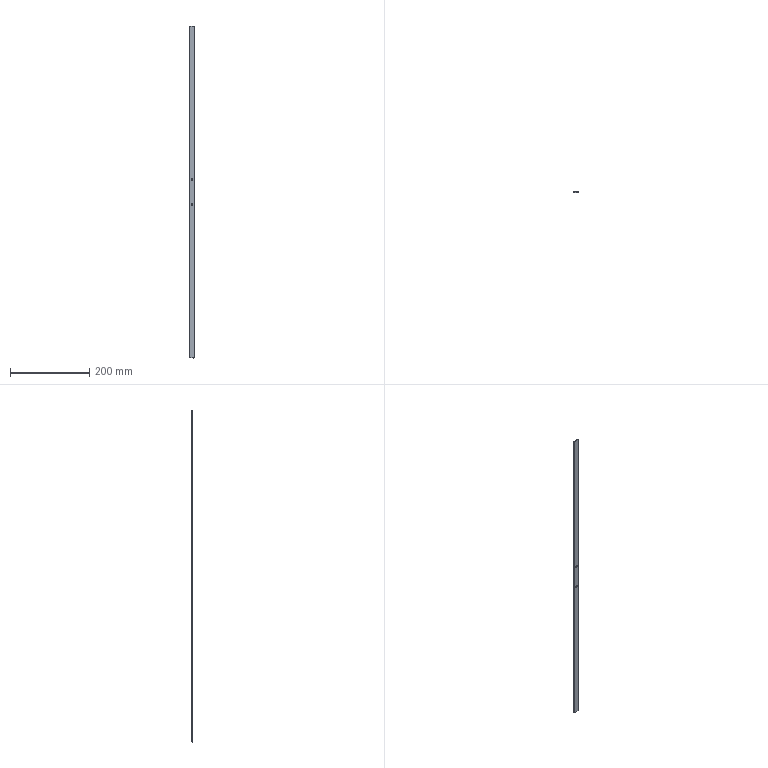Part | SolidWorks | features 3DProfileFeature 1, Extrusion 1, HoleWzd 1, ICE 1 | 1 solid | 18 faces | box 12 x 3 x 840 mm | volume 21761 mm3 | plane 10 | cylinder 8 | commonest cylinder face diameters 5 x8
STEP:
#1=CARTESIAN_POINT('',(-25.901,23.125,386.5));
#2=VERTEX_POINT('',#1);
#3=CARTESIAN_POINT('',(-25.901,23.125,391.5));
#4=VERTEX_POINT('',#3);
#5=CARTESIAN_POINT('',(-25.901,23.125,389.));
#6=DIRECTION('',(0.,1.,0.));
#7=DIRECTION('',(0.,0.,1.));
#8=AXIS2_PLACEMENT_3D('',#5,#6,#7);
#9=CIRCLE('',#8,2.5);
#10=EDGE_CURVE('',#2,#4,#9,.T.);
#11=ORIENTED_EDGE('',*,*,#10,.F.);
#12=CARTESIAN_POINT('',(-25.901,24.125,386.5));
#13=VERTEX_POINT('',#12);
#14=CARTESIAN_POINT('',(-25.901,24.125,386.5));
#15=DIRECTION('',(0.,1.,0.));
#16=VECTOR('',#15,1000.);
#17=LINE('',#14,#16);
#18=EDGE_CURVE('',#2,#13,#17,.T.);
#19=ORIENTED_EDGE('',*,*,#18,.T.);
#20=CARTESIAN_POINT('',(-25.901,24.125,391.5));
#21=VERTEX_POINT('',#20);
#22=CARTESIAN_POINT('',(-25.901,24.125,389.));
#23=DIRECTION('',(0.,1.,0.));
#24=DIRECTION('',(0.,0.,1.));
#25=AXIS2_PLACEMENT_3D('',#22,#23,#24);
#26=CIRCLE('',#25,2.5);
#27=EDGE_CURVE('',#13,#21,#26,.T.);
#28=ORIENTED_EDGE('',*,*,#27,.T.);
#29=CARTESIAN_POINT('',(-25.901,24.125,391.5));
#30=DIRECTION('',(0.,1.,0.));
#31=VECTOR('',#30,1000.);
#32=LINE('',#29,#31);
#33=EDGE_CURVE('',#4,#21,#32,.T.);
#34=ORIENTED_EDGE('',*,*,#33,.F.);
#35=EDGE_LOOP('',(#11,#19,#28,#34));
#36=FACE_OUTER_BOUND('',#35,.T.);
#37=CARTESIAN_POINT('',(-25.901,24.125,389.));
#38=DIRECTION('',(0.,1.,0.));
#39=DIRECTION('',(0.,0.,1.));
#40=AXIS2_PLACEMENT_3D('',#37,#38,#39);
#41=CYLINDRICAL_SURFACE('',#40,2.5);
#42=ADVANCED_FACE('',(#36),#41,.F.);
#43=CARTESIAN_POINT('',(-25.901,21.125,386.5));
#44=VERTEX_POINT('',#43);
#45=CARTESIAN_POINT('',(-25.901,21.125,391.5));
#46=VERTEX_POINT('',#45);
#47=CARTESIAN_POINT('',(-25.901,21.125,389.));
#48=DIRECTION('',(0.,1.,0.));
#49=DIRECTION('',(0.,0.,1.));
#50=AXIS2_PLACEMENT_3D('',#47,#48,#49);
#51=CIRCLE('',#50,2.5);
#52=EDGE_CURVE('',#44,#46,#51,.T.);
#53=ORIENTED_EDGE('',*,*,#52,.F.);
#54=CARTESIAN_POINT('',(-25.901,22.125,386.5));
#55=VERTEX_POINT('',#54);
#56=CARTESIAN_POINT('',(-25.901,24.125,386.5));
#57=DIRECTION('',(0.,1.,0.));
#58=VECTOR('',#57,1000.);
#59=LINE('',#56,#58);
#60=EDGE_CURVE('',#44,#55,#59,.T.);
#61=ORIENTED_EDGE('',*,*,#60,.T.);
#62=CARTESIAN_POINT('',(-25.901,22.125,391.5));
#63=VERTEX_POINT('',#62);
#64=CARTESIAN_POINT('',(-25.901,22.125,389.));
#65=DIRECTION('',(0.,-1.,0.));
#66=DIRECTION('',(0.,0.,-1.));
#67=AXIS2_PLACEMENT_3D('',#64,#65,#66);
#68=CIRCLE('',#67,2.5);
#69=EDGE_CURVE('',#63,#55,#68,.T.);
#70=ORIENTED_EDGE('',*,*,#69,.F.);
#71=CARTESIAN_POINT('',(-25.901,24.125,391.5));
#72=DIRECTION('',(0.,1.,0.));
#73=VECTOR('',#72,1000.);
#74=LINE('',#71,#73);
#75=EDGE_CURVE('',#46,#63,#74,.T.);
#76=ORIENTED_EDGE('',*,*,#75,.F.);
#77=EDGE_LOOP('',(#53,#61,#70,#76));
#78=FACE_OUTER_BOUND('',#77,.T.);
#79=CARTESIAN_POINT('',(-25.901,24.125,389.));
#80=DIRECTION('',(0.,1.,0.));
#81=DIRECTION('',(0.,0.,1.));
#82=AXIS2_PLACEMENT_3D('',#79,#80,#81);
#83=CYLINDRICAL_SURFACE('',#82,2.5);
#84=ADVANCED_FACE('',(#78),#83,.F.);
#85=CARTESIAN_POINT('',(-25.901,21.125,448.5));
#86=VERTEX_POINT('',#85);
#87=CARTESIAN_POINT('',(-25.901,21.125,453.5));
#88=VERTEX_POINT('',#87);
#89=CARTESIAN_POINT('',(-25.901,21.125,451.));
#90=DIRECTION('',(0.,1.,0.));
#91=DIRECTION('',(0.,0.,1.));
#92=AXIS2_PLACEMENT_3D('',#89,#90,#91);
#93=CIRCLE('',#92,2.5);
#94=EDGE_CURVE('',#86,#88,#93,.T.);
#95=ORIENTED_EDGE('',*,*,#94,.F.);
#96=CARTESIAN_POINT('',(-25.901,22.125,448.5));
#97=VERTEX_POINT('',#96);
#98=CARTESIAN_POINT('',(-25.901,24.125,448.5));
#99=DIRECTION('',(0.,1.,0.));
#100=VECTOR('',#99,1000.);
#101=LINE('',#98,#100);
#102=EDGE_CURVE('',#86,#97,#101,.T.);
#103=ORIENTED_EDGE('',*,*,#102,.T.);
#104=CARTESIAN_POINT('',(-25.901,22.125,453.5));
#105=VERTEX_POINT('',#104);
#106=CARTESIAN_POINT('',(-25.901,22.125,451.));
#107=DIRECTION('',(0.,-1.,0.));
#108=DIRECTION('',(0.,0.,-1.));
#109=AXIS2_PLACEMENT_3D('',#106,#107,#108);
#110=CIRCLE('',#109,2.5);
#111=EDGE_CURVE('',#105,#97,#110,.T.);
#112=ORIENTED_EDGE('',*,*,#111,.F.);
#113=CARTESIAN_POINT('',(-25.901,24.125,453.5));
#114=DIRECTION('',(0.,1.,0.));
#115=VECTOR('',#114,1000.);
#116=LINE('',#113,#115);
#117=EDGE_CURVE('',#88,#105,#116,.T.);
#118=ORIENTED_EDGE('',*,*,#117,.F.);
#119=EDGE_LOOP('',(#95,#103,#112,#118));
#120=FACE_OUTER_BOUND('',#119,.T.);
#121=CARTESIAN_POINT('',(-25.901,24.125,451.));
#122=DIRECTION('',(0.,1.,0.));
#123=DIRECTION('',(0.,0.,1.));
#124=AXIS2_PLACEMENT_3D('',#121,#122,#123);
#125=CYLINDRICAL_SURFACE('',#124,2.5);
#126=ADVANCED_FACE('',(#120),#125,.F.);
#127=CARTESIAN_POINT('',(-25.901,23.125,448.5));
#128=VERTEX_POINT('',#127);
#129=CARTESIAN_POINT('',(-25.901,23.125,453.5));
#130=VERTEX_POINT('',#129);
#131=CARTESIAN_POINT('',(-25.901,23.125,451.));
#132=DIRECTION('',(0.,1.,0.));
#133=DIRECTION('',(0.,0.,1.));
#134=AXIS2_PLACEMENT_3D('',#131,#132,#133);
#135=CIRCLE('',#134,2.5);
#136=EDGE_CURVE('',#128,#130,#135,.T.);
#137=ORIENTED_EDGE('',*,*,#136,.F.);
#138=CARTESIAN_POINT('',(-25.901,24.125,448.5));
#139=VERTEX_POINT('',#138);
#140=CARTESIAN_POINT('',(-25.901,24.125,448.5));
#141=DIRECTION('',(0.,1.,0.));
#142=VECTOR('',#141,1000.);
#143=LINE('',#140,#142);
#144=EDGE_CURVE('',#128,#139,#143,.T.);
#145=ORIENTED_EDGE('',*,*,#144,.T.);
#146=CARTESIAN_POINT('',(-25.901,24.125,453.5));
#147=VERTEX_POINT('',#146);
#148=CARTESIAN_POINT('',(-25.901,24.125,451.));
#149=DIRECTION('',(0.,1.,0.));
#150=DIRECTION('',(0.,0.,1.));
#151=AXIS2_PLACEMENT_3D('',#148,#149,#150);
#152=CIRCLE('',#151,2.5);
#153=EDGE_CURVE('',#139,#147,#152,.T.);
#154=ORIENTED_EDGE('',*,*,#153,.T.);
#155=CARTESIAN_POINT('',(-25.901,24.125,453.5));
#156=DIRECTION('',(0.,1.,0.));
#157=VECTOR('',#156,1000.);
#158=LINE('',#155,#157);
#159=EDGE_CURVE('',#130,#147,#158,.T.);
#160=ORIENTED_EDGE('',*,*,#159,.F.);
#161=EDGE_LOOP('',(#137,#145,#154,#160));
#162=FACE_OUTER_BOUND('',#161,.T.);
#163=CARTESIAN_POINT('',(-25.901,24.125,451.));
#164=DIRECTION('',(0.,1.,0.));
#165=DIRECTION('',(0.,0.,1.));
#166=AXIS2_PLACEMENT_3D('',#163,#164,#165);
#167=CYLINDRICAL_SURFACE('',#166,2.5);
#168=ADVANCED_FACE('',(#162),#167,.F.);
#169=CARTESIAN_POINT('',(-25.901,24.125,389.));
#170=DIRECTION('',(0.,1.,0.));
#171=DIRECTION('',(0.,0.,1.));
#172=AXIS2_PLACEMENT_3D('',#169,#170,#171);
#173=CIRCLE('',#172,2.5);
#174=EDGE_CURVE('',#21,#13,#173,.T.);
#175=ORIENTED_EDGE('',*,*,#174,.F.);
#176=ORIENTED_EDGE('',*,*,#27,.F.);
#177=EDGE_LOOP('',(#175,#176));
#178=FACE_BOUND('',#177,.T.);
#179=CARTESIAN_POINT('',(-19.901,24.125,0.));
#180=VERTEX_POINT('',#179);
#181=CARTESIAN_POINT('',(-31.901,24.125,0.));
#182=VERTEX_POINT('',#181);
#183=CARTESIAN_POINT('',(-31.901,24.125,0.));
#184=DIRECTION('',(-1.,0.,0.));
#185=VECTOR('',#184,1000.);
#186=LINE('',#183,#185);
#187=EDGE_CURVE('',#180,#182,#186,.T.);
#188=ORIENTED_EDGE('',*,*,#187,.T.);
#189=CARTESIAN_POINT('',(-31.901,24.125,840.));
#190=VERTEX_POINT('',#189);
#191=CARTESIAN_POINT('',(-31.901,24.125,840.));
#192=DIRECTION('',(0.,0.,-1.));
#193=VECTOR('',#192,1000.);
#194=LINE('',#191,#193);
#195=EDGE_CURVE('',#190,#182,#194,.T.);
#196=ORIENTED_EDGE('',*,*,#195,.F.);
#197=CARTESIAN_POINT('',(-19.901,24.125,840.));
#198=VERTEX_POINT('',#197);
#199=CARTESIAN_POINT('',(-31.901,24.125,840.));
#200=DIRECTION('',(-1.,0.,0.));
#201=VECTOR('',#200,1000.);
#202=LINE('',#199,#201);
#203=EDGE_CURVE('',#198,#190,#202,.T.);
#204=ORIENTED_EDGE('',*,*,#203,.F.);
#205=CARTESIAN_POINT('',(-19.901,24.125,840.));
#206=DIRECTION('',(0.,0.,-1.));
#207=VECTOR('',#206,1000.);
#208=LINE('',#205,#207);
#209=EDGE_CURVE('',#198,#180,#208,.T.);
#210=ORIENTED_EDGE('',*,*,#209,.T.);
#211=EDGE_LOOP('',(#188,#196,#204,#210));
#212=FACE_OUTER_BOUND('',#211,.T.);
#213=CARTESIAN_POINT('',(-25.901,24.125,451.));
#214=DIRECTION('',(0.,1.,0.));
#215=DIRECTION('',(0.,0.,1.));
#216=AXIS2_PLACEMENT_3D('',#213,#214,#215);
#217=CIRCLE('',#216,2.5);
#218=EDGE_CURVE('',#147,#139,#217,.T.);
#219=ORIENTED_EDGE('',*,*,#218,.F.);
#220=ORIENTED_EDGE('',*,*,#153,.F.);
#221=EDGE_LOOP('',(#219,#220));
#222=FACE_BOUND('',#221,.T.);
#223=CARTESIAN_POINT('',(-31.901,24.125,840.));
#224=DIRECTION('',(0.,-1.,0.));
#225=DIRECTION('',(0.,0.,-1.));
#226=AXIS2_PLACEMENT_3D('',#223,#224,#225);
#227=PLANE('',#226);
#228=ADVANCED_FACE('',(#178,#212,#222),#227,.F.);
#229=CARTESIAN_POINT('',(-31.901,21.125,0.));
#230=VERTEX_POINT('',#229);
#231=CARTESIAN_POINT('',(-31.901,21.125,0.));
#232=DIRECTION('',(0.,-1.,0.));
#233=VECTOR('',#232,1000.);
#234=LINE('',#231,#233);
#235=EDGE_CURVE('',#182,#230,#234,.T.);
#236=ORIENTED_EDGE('',*,*,#235,.T.);
#237=CARTESIAN_POINT('',(-31.901,21.125,840.));
#238=VERTEX_POINT('',#237);
#239=CARTESIAN_POINT('',(-31.901,21.125,840.));
#240=DIRECTION('',(0.,0.,-1.));
#241=VECTOR('',#240,1000.);
#242=LINE('',#239,#241);
#243=EDGE_CURVE('',#238,#230,#242,.T.);
#244=ORIENTED_EDGE('',*,*,#243,.F.);
#245=CARTESIAN_POINT('',(-31.901,21.125,840.));
#246=DIRECTION('',(0.,-1.,0.));
#247=VECTOR('',#246,1000.);
#248=LINE('',#245,#247);
#249=EDGE_CURVE('',#190,#238,#248,.T.);
#250=ORIENTED_EDGE('',*,*,#249,.F.);
#251=ORIENTED_EDGE('',*,*,#195,.T.);
#252=EDGE_LOOP('',(#236,#244,#250,#251));
#253=FACE_OUTER_BOUND('',#252,.T.);
#254=CARTESIAN_POINT('',(-31.901,21.125,840.));
#255=DIRECTION('',(1.,0.,0.));
#256=DIRECTION('',(0.,0.,-1.));
#257=AXIS2_PLACEMENT_3D('',#254,#255,#256);
#258=PLANE('',#257);
#259=ADVANCED_FACE('',(#253),#258,.F.);
#260=CARTESIAN_POINT('',(-25.901,21.125,389.));
#261=DIRECTION('',(0.,1.,0.));
#262=DIRECTION('',(0.,0.,1.));
#263=AXIS2_PLACEMENT_3D('',#260,#261,#262);
#264=CIRCLE('',#263,2.5);
#265=EDGE_CURVE('',#46,#44,#264,.T.);
#266=ORIENTED_EDGE('',*,*,#265,.T.);
#267=ORIENTED_EDGE('',*,*,#52,.T.);
#268=EDGE_LOOP('',(#266,#267));
#269=FACE_BOUND('',#268,.T.);
#270=CARTESIAN_POINT('',(-25.901,21.125,451.));
#271=DIRECTION('',(0.,1.,0.));
#272=DIRECTION('',(0.,0.,1.));
#273=AXIS2_PLACEMENT_3D('',#270,#271,#272);
#274=CIRCLE('',#273,2.5);
#275=EDGE_CURVE('',#88,#86,#274,.T.);
#276=ORIENTED_EDGE('',*,*,#275,.T.);
#277=ORIENTED_EDGE('',*,*,#94,.T.);
#278=EDGE_LOOP('',(#276,#277));
#279=FACE_BOUND('',#278,.T.);
#280=CARTESIAN_POINT('',(-19.901,21.125,0.));
#281=VERTEX_POINT('',#280);
#282=CARTESIAN_POINT('',(-19.901,21.125,0.));
#283=DIRECTION('',(1.,0.,0.));
#284=VECTOR('',#283,1000.);
#285=LINE('',#282,#284);
#286=EDGE_CURVE('',#230,#281,#285,.T.);
#287=ORIENTED_EDGE('',*,*,#286,.T.);
#288=CARTESIAN_POINT('',(-19.901,21.125,840.));
#289=VERTEX_POINT('',#288);
#290=CARTESIAN_POINT('',(-19.901,21.125,840.));
#291=DIRECTION('',(0.,0.,-1.));
#292=VECTOR('',#291,1000.);
#293=LINE('',#290,#292);
#294=EDGE_CURVE('',#289,#281,#293,.T.);
#295=ORIENTED_EDGE('',*,*,#294,.F.);
#296=CARTESIAN_POINT('',(-19.901,21.125,840.));
#297=DIRECTION('',(1.,0.,0.));
#298=VECTOR('',#297,1000.);
#299=LINE('',#296,#298);
#300=EDGE_CURVE('',#238,#289,#299,.T.);
#301=ORIENTED_EDGE('',*,*,#300,.F.);
#302=ORIENTED_EDGE('',*,*,#243,.T.);
#303=EDGE_LOOP('',(#287,#295,#301,#302));
#304=FACE_OUTER_BOUND('',#303,.T.);
#305=CARTESIAN_POINT('',(-19.901,21.125,840.));
#306=DIRECTION('',(0.,1.,0.));
#307=DIRECTION('',(0.,0.,1.));
#308=AXIS2_PLACEMENT_3D('',#305,#306,#307);
#309=PLANE('',#308);
#310=ADVANCED_FACE('',(#269,#279,#304),#309,.F.);
#311=CARTESIAN_POINT('',(-19.901,24.125,0.));
#312=DIRECTION('',(0.,1.,0.));
#313=VECTOR('',#312,1000.);
#314=LINE('',#311,#313);
#315=EDGE_CURVE('',#281,#180,#314,.T.);
#316=ORIENTED_EDGE('',*,*,#315,.T.);
#317=ORIENTED_EDGE('',*,*,#209,.F.);
#318=CARTESIAN_POINT('',(-19.901,24.125,840.));
#319=DIRECTION('',(0.,1.,0.));
#320=VECTOR('',#319,1000.);
#321=LINE('',#318,#320);
#322=EDGE_CURVE('',#289,#198,#321,.T.);
#323=ORIENTED_EDGE('',*,*,#322,.F.);
#324=ORIENTED_EDGE('',*,*,#294,.T.);
#325=EDGE_LOOP('',(#316,#317,#323,#324));
#326=FACE_OUTER_BOUND('',#325,.T.);
#327=CARTESIAN_POINT('',(-19.901,24.125,840.));
#328=DIRECTION('',(-1.,0.,0.));
#329=DIRECTION('',(0.,0.,1.));
#330=AXIS2_PLACEMENT_3D('',#327,#328,#329);
#331=PLANE('',#330);
#332=ADVANCED_FACE('',(#326),#331,.F.);
#333=CARTESIAN_POINT('',(-30.901,22.125,840.));
#334=VERTEX_POINT('',#333);
#335=CARTESIAN_POINT('',(-20.901,22.125,840.));
#336=VERTEX_POINT('',#335);
#337=CARTESIAN_POINT('',(-20.901,22.125,840.));
#338=DIRECTION('',(1.,0.,0.));
#339=VECTOR('',#338,1000.);
#340=LINE('',#337,#339);
#341=EDGE_CURVE('',#334,#336,#340,.T.);
#342=ORIENTED_EDGE('',*,*,#341,.F.);
#343=CARTESIAN_POINT('',(-30.901,23.125,840.));
#344=VERTEX_POINT('',#343);
#345=CARTESIAN_POINT('',(-30.901,22.125,840.));
#346=DIRECTION('',(0.,-1.,0.));
#347=VECTOR('',#346,1000.);
#348=LINE('',#345,#347);
#349=EDGE_CURVE('',#344,#334,#348,.T.);
#350=ORIENTED_EDGE('',*,*,#349,.F.);
#351=CARTESIAN_POINT('',(-20.901,23.125,840.));
#352=VERTEX_POINT('',#351);
#353=CARTESIAN_POINT('',(-30.901,23.125,840.));
#354=DIRECTION('',(-1.,0.,0.));
#355=VECTOR('',#354,1000.);
#356=LINE('',#353,#355);
#357=EDGE_CURVE('',#352,#344,#356,.T.);
#358=ORIENTED_EDGE('',*,*,#357,.F.);
#359=CARTESIAN_POINT('',(-20.901,23.125,840.));
#360=DIRECTION('',(0.,1.,0.));
#361=VECTOR('',#360,1000.);
#362=LINE('',#359,#361);
#363=EDGE_CURVE('',#336,#352,#362,.T.);
#364=ORIENTED_EDGE('',*,*,#363,.F.);
#365=EDGE_LOOP('',(#342,#350,#358,#364));
#366=FACE_BOUND('',#365,.T.);
#367=ORIENTED_EDGE('',*,*,#249,.T.);
#368=ORIENTED_EDGE('',*,*,#300,.T.);
#369=ORIENTED_EDGE('',*,*,#322,.T.);
#370=ORIENTED_EDGE('',*,*,#203,.T.);
#371=EDGE_LOOP('',(#367,#368,#369,#370));
#372=FACE_OUTER_BOUND('',#371,.T.);
#373=CARTESIAN_POINT('',(0.,0.,840.));
#374=DIRECTION('',(0.,0.,-1.));
#375=DIRECTION('',(-1.,0.,0.));
#376=AXIS2_PLACEMENT_3D('',#373,#374,#375);
#377=PLANE('',#376);
#378=ADVANCED_FACE('',(#366,#372),#377,.F.);
#379=CARTESIAN_POINT('',(-30.901,23.125,0.));
#380=VERTEX_POINT('',#379);
#381=CARTESIAN_POINT('',(-30.901,22.125,0.));
#382=VERTEX_POINT('',#381);
#383=CARTESIAN_POINT('',(-30.901,22.125,0.));
#384=DIRECTION('',(0.,-1.,0.));
#385=VECTOR('',#384,1000.);
#386=LINE('',#383,#385);
#387=EDGE_CURVE('',#380,#382,#386,.T.);
#388=ORIENTED_EDGE('',*,*,#387,.T.);
#389=CARTESIAN_POINT('',(-20.901,22.125,0.));
#390=VERTEX_POINT('',#389);
#391=CARTESIAN_POINT('',(-20.901,22.125,0.));
#392=DIRECTION('',(1.,0.,0.));
#393=VECTOR('',#392,1000.);
#394=LINE('',#391,#393);
#395=EDGE_CURVE('',#382,#390,#394,.T.);
#396=ORIENTED_EDGE('',*,*,#395,.T.);
#397=CARTESIAN_POINT('',(-20.901,23.125,0.));
#398=VERTEX_POINT('',#397);
#399=CARTESIAN_POINT('',(-20.901,23.125,0.));
#400=DIRECTION('',(0.,1.,0.));
#401=VECTOR('',#400,1000.);
#402=LINE('',#399,#401);
#403=EDGE_CURVE('',#390,#398,#402,.T.);
#404=ORIENTED_EDGE('',*,*,#403,.T.);
#405=CARTESIAN_POINT('',(-30.901,23.125,0.));
#406=DIRECTION('',(-1.,0.,0.));
#407=VECTOR('',#406,1000.);
#408=LINE('',#405,#407);
#409=EDGE_CURVE('',#398,#380,#408,.T.);
#410=ORIENTED_EDGE('',*,*,#409,.T.);
#411=EDGE_LOOP('',(#388,#396,#404,#410));
#412=FACE_BOUND('',#411,.T.);
#413=ORIENTED_EDGE('',*,*,#235,.F.);
#414=ORIENTED_EDGE('',*,*,#187,.F.);
#415=ORIENTED_EDGE('',*,*,#315,.F.);
#416=ORIENTED_EDGE('',*,*,#286,.F.);
#417=EDGE_LOOP('',(#413,#414,#415,#416));
#418=FACE_OUTER_BOUND('',#417,.T.);
#419=CARTESIAN_POINT('',(0.,0.,0.));
#420=DIRECTION('',(0.,0.,-1.));
#421=DIRECTION('',(-1.,0.,0.));
#422=AXIS2_PLACEMENT_3D('',#419,#420,#421);
#423=PLANE('',#422);
#424=ADVANCED_FACE('',(#412,#418),#423,.T.);
#425=ORIENTED_EDGE('',*,*,#349,.T.);
#426=CARTESIAN_POINT('',(-30.901,22.125,0.));
#427=DIRECTION('',(0.,0.,1.));
#428=VECTOR('',#427,1000.);
#429=LINE('',#426,#428);
#430=EDGE_CURVE('',#382,#334,#429,.T.);
#431=ORIENTED_EDGE('',*,*,#430,.F.);
#432=ORIENTED_EDGE('',*,*,#387,.F.);
#433=CARTESIAN_POINT('',(-30.901,23.125,0.));
#434=DIRECTION('',(0.,0.,1.));
#435=VECTOR('',#434,1000.);
#436=LINE('',#433,#435);
#437=EDGE_CURVE('',#380,#344,#436,.T.);
#438=ORIENTED_EDGE('',*,*,#437,.T.);
#439=EDGE_LOOP('',(#425,#431,#432,#438));
#440=FACE_OUTER_BOUND('',#439,.T.);
#441=CARTESIAN_POINT('',(-30.901,22.125,0.));
#442=DIRECTION('',(-1.,0.,0.));
#443=DIRECTION('',(0.,0.,1.));
#444=AXIS2_PLACEMENT_3D('',#441,#442,#443);
#445=PLANE('',#444);
#446=ADVANCED_FACE('',(#440),#445,.F.);
#447=CARTESIAN_POINT('',(-25.901,23.125,389.));
#448=DIRECTION('',(0.,1.,0.));
#449=DIRECTION('',(0.,0.,1.));
#450=AXIS2_PLACEMENT_3D('',#447,#448,#449);
#451=CIRCLE('',#450,2.5);
#452=EDGE_CURVE('',#4,#2,#451,.T.);
#453=ORIENTED_EDGE('',*,*,#452,.T.);
#454=ORIENTED_EDGE('',*,*,#10,.T.);
#455=EDGE_LOOP('',(#453,#454));
#456=FACE_BOUND('',#455,.T.);
#457=CARTESIAN_POINT('',(-25.901,23.125,451.));
#458=DIRECTION('',(0.,1.,0.));
#459=DIRECTION('',(0.,0.,1.));
#460=AXIS2_PLACEMENT_3D('',#457,#458,#459);
#461=CIRCLE('',#460,2.5);
#462=EDGE_CURVE('',#130,#128,#461,.T.);
#463=ORIENTED_EDGE('',*,*,#462,.T.);
#464=ORIENTED_EDGE('',*,*,#136,.T.);
#465=EDGE_LOOP('',(#463,#464));
#466=FACE_BOUND('',#465,.T.);
#467=ORIENTED_EDGE('',*,*,#357,.T.);
#468=ORIENTED_EDGE('',*,*,#437,.F.);
#469=ORIENTED_EDGE('',*,*,#409,.F.);
#470=CARTESIAN_POINT('',(-20.901,23.125,0.));
#471=DIRECTION('',(0.,0.,1.));
#472=VECTOR('',#471,1000.);
#473=LINE('',#470,#472);
#474=EDGE_CURVE('',#398,#352,#473,.T.);
#475=ORIENTED_EDGE('',*,*,#474,.T.);
#476=EDGE_LOOP('',(#467,#468,#469,#475));
#477=FACE_OUTER_BOUND('',#476,.T.);
#478=CARTESIAN_POINT('',(-30.901,23.125,0.));
#479=DIRECTION('',(0.,1.,0.));
#480=DIRECTION('',(0.,0.,1.));
#481=AXIS2_PLACEMENT_3D('',#478,#479,#480);
#482=PLANE('',#481);
#483=ADVANCED_FACE('',(#456,#466,#477),#482,.F.);
#484=ORIENTED_EDGE('',*,*,#363,.T.);
#485=ORIENTED_EDGE('',*,*,#474,.F.);
#486=ORIENTED_EDGE('',*,*,#403,.F.);
#487=CARTESIAN_POINT('',(-20.901,22.125,0.));
#488=DIRECTION('',(0.,0.,1.));
#489=VECTOR('',#488,1000.);
#490=LINE('',#487,#489);
#491=EDGE_CURVE('',#390,#336,#490,.T.);
#492=ORIENTED_EDGE('',*,*,#491,.T.);
#493=EDGE_LOOP('',(#484,#485,#486,#492));
#494=FACE_OUTER_BOUND('',#493,.T.);
#495=CARTESIAN_POINT('',(-20.901,23.125,0.));
#496=DIRECTION('',(1.,0.,0.));
#497=DIRECTION('',(0.,0.,-1.));
#498=AXIS2_PLACEMENT_3D('',#495,#496,#497);
#499=PLANE('',#498);
#500=ADVANCED_FACE('',(#494),#499,.F.);
#501=ORIENTED_EDGE('',*,*,#69,.T.);
#502=CARTESIAN_POINT('',(-25.901,22.125,389.));
#503=DIRECTION('',(0.,-1.,0.));
#504=DIRECTION('',(0.,0.,-1.));
#505=AXIS2_PLACEMENT_3D('',#502,#503,#504);
#506=CIRCLE('',#505,2.5);
#507=EDGE_CURVE('',#55,#63,#506,.T.);
#508=ORIENTED_EDGE('',*,*,#507,.T.);
#509=EDGE_LOOP('',(#501,#508));
#510=FACE_BOUND('',#509,.T.);
#511=ORIENTED_EDGE('',*,*,#111,.T.);
#512=CARTESIAN_POINT('',(-25.901,22.125,451.));
#513=DIRECTION('',(0.,-1.,0.));
#514=DIRECTION('',(0.,0.,-1.));
#515=AXIS2_PLACEMENT_3D('',#512,#513,#514);
#516=CIRCLE('',#515,2.5);
#517=EDGE_CURVE('',#97,#105,#516,.T.);
#518=ORIENTED_EDGE('',*,*,#517,.T.);
#519=EDGE_LOOP('',(#511,#518));
#520=FACE_BOUND('',#519,.T.);
#521=ORIENTED_EDGE('',*,*,#341,.T.);
#522=ORIENTED_EDGE('',*,*,#491,.F.);
#523=ORIENTED_EDGE('',*,*,#395,.F.);
#524=ORIENTED_EDGE('',*,*,#430,.T.);
#525=EDGE_LOOP('',(#521,#522,#523,#524));
#526=FACE_OUTER_BOUND('',#525,.T.);
#527=CARTESIAN_POINT('',(-20.901,22.125,0.));
#528=DIRECTION('',(0.,-1.,0.));
#529=DIRECTION('',(0.,0.,-1.));
#530=AXIS2_PLACEMENT_3D('',#527,#528,#529);
#531=PLANE('',#530);
#532=ADVANCED_FACE('',(#510,#520,#526),#531,.F.);
#533=ORIENTED_EDGE('',*,*,#144,.F.);
#534=ORIENTED_EDGE('',*,*,#462,.F.);
#535=ORIENTED_EDGE('',*,*,#159,.T.);
#536=ORIENTED_EDGE('',*,*,#218,.T.);
#537=EDGE_LOOP('',(#533,#534,#535,#536));
#538=FACE_OUTER_BOUND('',#537,.T.);
#539=CARTESIAN_POINT('',(-25.901,24.125,451.));
#540=DIRECTION('',(0.,1.,0.));
#541=DIRECTION('',(0.,0.,1.));
#542=AXIS2_PLACEMENT_3D('',#539,#540,#541);
#543=CYLINDRICAL_SURFACE('',#542,2.5);
#544=ADVANCED_FACE('',(#538),#543,.F.);
#545=ORIENTED_EDGE('',*,*,#102,.F.);
#546=ORIENTED_EDGE('',*,*,#275,.F.);
#547=ORIENTED_EDGE('',*,*,#117,.T.);
#548=ORIENTED_EDGE('',*,*,#517,.F.);
#549=EDGE_LOOP('',(#545,#546,#547,#548));
#550=FACE_OUTER_BOUND('',#549,.T.);
#551=CARTESIAN_POINT('',(-25.901,24.125,451.));
#552=DIRECTION('',(0.,1.,0.));
#553=DIRECTION('',(0.,0.,1.));
#554=AXIS2_PLACEMENT_3D('',#551,#552,#553);
#555=CYLINDRICAL_SURFACE('',#554,2.5);
#556=ADVANCED_FACE('',(#550),#555,.F.);
#557=ORIENTED_EDGE('',*,*,#60,.F.);
#558=ORIENTED_EDGE('',*,*,#265,.F.);
#559=ORIENTED_EDGE('',*,*,#75,.T.);
#560=ORIENTED_EDGE('',*,*,#507,.F.);
#561=EDGE_LOOP('',(#557,#558,#559,#560));
#562=FACE_OUTER_BOUND('',#561,.T.);
#563=CARTESIAN_POINT('',(-25.901,24.125,389.));
#564=DIRECTION('',(0.,1.,0.));
#565=DIRECTION('',(0.,0.,1.));
#566=AXIS2_PLACEMENT_3D('',#563,#564,#565);
#567=CYLINDRICAL_SURFACE('',#566,2.5);
#568=ADVANCED_FACE('',(#562),#567,.F.);
#569=ORIENTED_EDGE('',*,*,#18,.F.);
#570=ORIENTED_EDGE('',*,*,#452,.F.);
#571=ORIENTED_EDGE('',*,*,#33,.T.);
#572=ORIENTED_EDGE('',*,*,#174,.T.);
#573=EDGE_LOOP('',(#569,#570,#571,#572));
#574=FACE_OUTER_BOUND('',#573,.T.);
#575=CARTESIAN_POINT('',(-25.901,24.125,389.));
#576=DIRECTION('',(0.,1.,0.));
#577=DIRECTION('',(0.,0.,1.));
#578=AXIS2_PLACEMENT_3D('',#575,#576,#577);
#579=CYLINDRICAL_SURFACE('',#578,2.5);
#580=ADVANCED_FACE('',(#574),#579,.F.);
#581=CLOSED_SHELL('',(#42,#84,#126,#168,#228,#259,#310,#332,#378,#424,#446,#483,#500,#532,#544,#556,#568,#580));
#582=MANIFOLD_SOLID_BREP('',#581);
#583=CARTESIAN_POINT('',(0.,0.,0.));
#584=DIRECTION('',(0.,0.,1.));
#585=DIRECTION('',(1.,0.,0.));
#586=AXIS2_PLACEMENT_3D('',#583,#584,#585);
#587=(LENGTH_UNIT()NAMED_UNIT(*)SI_UNIT(.MILLI.,.METRE.));
#588=UNCERTAINTY_MEASURE_WITH_UNIT(LENGTH_MEASURE(0.00001),#587,'','');
#589=(NAMED_UNIT(*)PLANE_ANGLE_UNIT()SI_UNIT($,.RADIAN.));
#590=(NAMED_UNIT(*)SI_UNIT($,.STERADIAN.)SOLID_ANGLE_UNIT());
#591=(GEOMETRIC_REPRESENTATION_CONTEXT(3)GLOBAL_UNCERTAINTY_ASSIGNED_CONTEXT((#588))GLOBAL_UNIT_ASSIGNED_CONTEXT((#587,#589,#590))REPRESENTATION_CONTEXT('',''));
#592=ADVANCED_BREP_SHAPE_REPRESENTATION('',(#582,#586),#591);